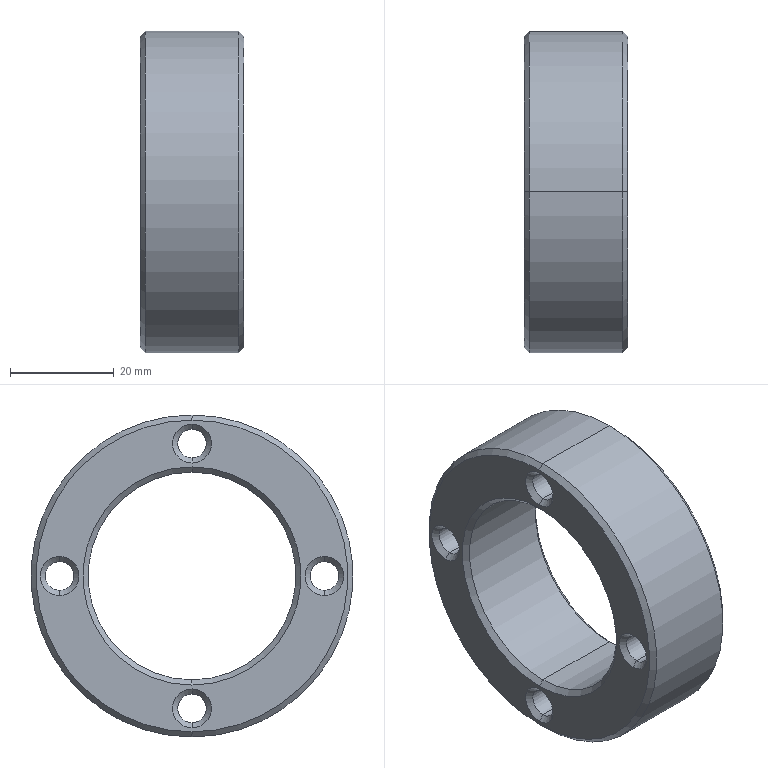Part | SolidWorks | features BaseBody 1 | 1 solid | 38 faces | box 20 x 62 x 62 mm | volume 32950 mm3 | cone 24 | cylinder 12 | plane 2 | commonest cylinder face diameters 5.5 x8 40 x2 62 x2
STEP:
#1=CARTESIAN_POINT('',(1.,0.,-28.25));
#2=VERTEX_POINT('',#1);
#3=CARTESIAN_POINT('',(1.,0.,-22.75));
#4=VERTEX_POINT('',#3);
#5=CARTESIAN_POINT('',(1.,0.,-25.5));
#6=DIRECTION('',(-1.,0.,0.));
#7=DIRECTION('',(0.,0.,-1.));
#8=AXIS2_PLACEMENT_3D('',#5,#6,#7);
#9=CIRCLE('',#8,2.75);
#10=EDGE_CURVE('',#2,#4,#9,.T.);
#11=ORIENTED_EDGE('',*,*,#10,.F.);
#12=CARTESIAN_POINT('',(0.,0.,-29.25));
#13=VERTEX_POINT('',#12);
#14=CARTESIAN_POINT('',(1.,0.,-28.25));
#15=DIRECTION('',(-0.7071,0.,-0.7071));
#16=VECTOR('',#15,1000.);
#17=LINE('',#14,#16);
#18=EDGE_CURVE('',#2,#13,#17,.T.);
#19=ORIENTED_EDGE('',*,*,#18,.T.);
#20=CARTESIAN_POINT('',(0.,0.,-21.75));
#21=VERTEX_POINT('',#20);
#22=CARTESIAN_POINT('',(0.,0.,-25.5));
#23=DIRECTION('',(1.,0.,0.));
#24=DIRECTION('',(0.,0.,-1.));
#25=AXIS2_PLACEMENT_3D('',#22,#23,#24);
#26=CIRCLE('',#25,3.75);
#27=EDGE_CURVE('',#21,#13,#26,.T.);
#28=ORIENTED_EDGE('',*,*,#27,.F.);
#29=CARTESIAN_POINT('',(1.,0.,-22.75));
#30=DIRECTION('',(-0.7071,0.,0.7071));
#31=VECTOR('',#30,1000.);
#32=LINE('',#29,#31);
#33=EDGE_CURVE('',#4,#21,#32,.T.);
#34=ORIENTED_EDGE('',*,*,#33,.F.);
#35=EDGE_LOOP('',(#11,#19,#28,#34));
#36=FACE_OUTER_BOUND('',#35,.T.);
#37=CARTESIAN_POINT('',(1.,0.,-25.5));
#38=DIRECTION('',(-1.,0.,0.));
#39=DIRECTION('',(0.,0.,1.));
#40=AXIS2_PLACEMENT_3D('',#37,#38,#39);
#41=CONICAL_SURFACE('',#40,2.75,0.7854);
#42=ADVANCED_FACE('',(#36),#41,.F.);
#43=CARTESIAN_POINT('',(1.,-25.5,-2.75));
#44=VERTEX_POINT('',#43);
#45=CARTESIAN_POINT('',(1.,-25.5,2.75));
#46=VERTEX_POINT('',#45);
#47=CARTESIAN_POINT('',(1.,-25.5,0.));
#48=DIRECTION('',(-1.,0.,0.));
#49=DIRECTION('',(0.,0.,-1.));
#50=AXIS2_PLACEMENT_3D('',#47,#48,#49);
#51=CIRCLE('',#50,2.75);
#52=EDGE_CURVE('',#44,#46,#51,.T.);
#53=ORIENTED_EDGE('',*,*,#52,.F.);
#54=CARTESIAN_POINT('',(0.,-25.5,-3.75));
#55=VERTEX_POINT('',#54);
#56=CARTESIAN_POINT('',(1.,-25.5,-2.75));
#57=DIRECTION('',(-0.7071,0.,-0.7071));
#58=VECTOR('',#57,1000.);
#59=LINE('',#56,#58);
#60=EDGE_CURVE('',#44,#55,#59,.T.);
#61=ORIENTED_EDGE('',*,*,#60,.T.);
#62=CARTESIAN_POINT('',(0.,-25.5,3.75));
#63=VERTEX_POINT('',#62);
#64=CARTESIAN_POINT('',(0.,-25.5,0.));
#65=DIRECTION('',(1.,0.,0.));
#66=DIRECTION('',(0.,0.,-1.));
#67=AXIS2_PLACEMENT_3D('',#64,#65,#66);
#68=CIRCLE('',#67,3.75);
#69=EDGE_CURVE('',#63,#55,#68,.T.);
#70=ORIENTED_EDGE('',*,*,#69,.F.);
#71=CARTESIAN_POINT('',(1.,-25.5,2.75));
#72=DIRECTION('',(-0.7071,0.,0.7071));
#73=VECTOR('',#72,1000.);
#74=LINE('',#71,#73);
#75=EDGE_CURVE('',#46,#63,#74,.T.);
#76=ORIENTED_EDGE('',*,*,#75,.F.);
#77=EDGE_LOOP('',(#53,#61,#70,#76));
#78=FACE_OUTER_BOUND('',#77,.T.);
#79=CARTESIAN_POINT('',(1.,-25.5,0.));
#80=DIRECTION('',(-1.,0.,0.));
#81=DIRECTION('',(0.,0.,1.));
#82=AXIS2_PLACEMENT_3D('',#79,#80,#81);
#83=CONICAL_SURFACE('',#82,2.75,0.7854);
#84=ADVANCED_FACE('',(#78),#83,.F.);
#85=CARTESIAN_POINT('',(1.,0.,22.75));
#86=VERTEX_POINT('',#85);
#87=CARTESIAN_POINT('',(1.,0.,28.25));
#88=VERTEX_POINT('',#87);
#89=CARTESIAN_POINT('',(1.,0.,25.5));
#90=DIRECTION('',(-1.,0.,0.));
#91=DIRECTION('',(0.,0.,-1.));
#92=AXIS2_PLACEMENT_3D('',#89,#90,#91);
#93=CIRCLE('',#92,2.75);
#94=EDGE_CURVE('',#86,#88,#93,.T.);
#95=ORIENTED_EDGE('',*,*,#94,.F.);
#96=CARTESIAN_POINT('',(0.,0.,21.75));
#97=VERTEX_POINT('',#96);
#98=CARTESIAN_POINT('',(1.,0.,22.75));
#99=DIRECTION('',(-0.7071,0.,-0.7071));
#100=VECTOR('',#99,1000.);
#101=LINE('',#98,#100);
#102=EDGE_CURVE('',#86,#97,#101,.T.);
#103=ORIENTED_EDGE('',*,*,#102,.T.);
#104=CARTESIAN_POINT('',(0.,0.,29.25));
#105=VERTEX_POINT('',#104);
#106=CARTESIAN_POINT('',(0.,0.,25.5));
#107=DIRECTION('',(1.,0.,0.));
#108=DIRECTION('',(0.,0.,-1.));
#109=AXIS2_PLACEMENT_3D('',#106,#107,#108);
#110=CIRCLE('',#109,3.75);
#111=EDGE_CURVE('',#105,#97,#110,.T.);
#112=ORIENTED_EDGE('',*,*,#111,.F.);
#113=CARTESIAN_POINT('',(1.,0.,28.25));
#114=DIRECTION('',(-0.7071,0.,0.7071));
#115=VECTOR('',#114,1000.);
#116=LINE('',#113,#115);
#117=EDGE_CURVE('',#88,#105,#116,.T.);
#118=ORIENTED_EDGE('',*,*,#117,.F.);
#119=EDGE_LOOP('',(#95,#103,#112,#118));
#120=FACE_OUTER_BOUND('',#119,.T.);
#121=CARTESIAN_POINT('',(1.,0.,25.5));
#122=DIRECTION('',(-1.,0.,0.));
#123=DIRECTION('',(0.,0.,1.));
#124=AXIS2_PLACEMENT_3D('',#121,#122,#123);
#125=CONICAL_SURFACE('',#124,2.75,0.7854);
#126=ADVANCED_FACE('',(#120),#125,.F.);
#127=CARTESIAN_POINT('',(1.,25.5,-2.75));
#128=VERTEX_POINT('',#127);
#129=CARTESIAN_POINT('',(1.,25.5,2.75));
#130=VERTEX_POINT('',#129);
#131=CARTESIAN_POINT('',(1.,25.5,0.));
#132=DIRECTION('',(-1.,0.,0.));
#133=DIRECTION('',(0.,0.,-1.));
#134=AXIS2_PLACEMENT_3D('',#131,#132,#133);
#135=CIRCLE('',#134,2.75);
#136=EDGE_CURVE('',#128,#130,#135,.T.);
#137=ORIENTED_EDGE('',*,*,#136,.F.);
#138=CARTESIAN_POINT('',(0.,25.5,-3.75));
#139=VERTEX_POINT('',#138);
#140=CARTESIAN_POINT('',(1.,25.5,-2.75));
#141=DIRECTION('',(-0.7071,0.,-0.7071));
#142=VECTOR('',#141,1000.);
#143=LINE('',#140,#142);
#144=EDGE_CURVE('',#128,#139,#143,.T.);
#145=ORIENTED_EDGE('',*,*,#144,.T.);
#146=CARTESIAN_POINT('',(0.,25.5,3.75));
#147=VERTEX_POINT('',#146);
#148=CARTESIAN_POINT('',(0.,25.5,0.));
#149=DIRECTION('',(1.,0.,0.));
#150=DIRECTION('',(0.,0.,-1.));
#151=AXIS2_PLACEMENT_3D('',#148,#149,#150);
#152=CIRCLE('',#151,3.75);
#153=EDGE_CURVE('',#147,#139,#152,.T.);
#154=ORIENTED_EDGE('',*,*,#153,.F.);
#155=CARTESIAN_POINT('',(1.,25.5,2.75));
#156=DIRECTION('',(-0.7071,0.,0.7071));
#157=VECTOR('',#156,1000.);
#158=LINE('',#155,#157);
#159=EDGE_CURVE('',#130,#147,#158,.T.);
#160=ORIENTED_EDGE('',*,*,#159,.F.);
#161=EDGE_LOOP('',(#137,#145,#154,#160));
#162=FACE_OUTER_BOUND('',#161,.T.);
#163=CARTESIAN_POINT('',(1.,25.5,0.));
#164=DIRECTION('',(-1.,0.,0.));
#165=DIRECTION('',(0.,0.,1.));
#166=AXIS2_PLACEMENT_3D('',#163,#164,#165);
#167=CONICAL_SURFACE('',#166,2.75,0.7854);
#168=ADVANCED_FACE('',(#162),#167,.F.);
#169=CARTESIAN_POINT('',(0.,0.,30.));
#170=VERTEX_POINT('',#169);
#171=CARTESIAN_POINT('',(0.,0.,-30.));
#172=VERTEX_POINT('',#171);
#173=CARTESIAN_POINT('',(0.,0.,0.));
#174=DIRECTION('',(-1.,0.,0.));
#175=DIRECTION('',(0.,0.,-1.));
#176=AXIS2_PLACEMENT_3D('',#173,#174,#175);
#177=CIRCLE('',#176,30.);
#178=EDGE_CURVE('',#170,#172,#177,.T.);
#179=ORIENTED_EDGE('',*,*,#178,.F.);
#180=CARTESIAN_POINT('',(1.,0.,31.));
#181=VERTEX_POINT('',#180);
#182=CARTESIAN_POINT('',(1.,0.,31.));
#183=DIRECTION('',(0.7071,0.,0.7071));
#184=VECTOR('',#183,1000.);
#185=LINE('',#182,#184);
#186=EDGE_CURVE('',#170,#181,#185,.T.);
#187=ORIENTED_EDGE('',*,*,#186,.T.);
#188=CARTESIAN_POINT('',(1.,0.,-31.));
#189=VERTEX_POINT('',#188);
#190=CARTESIAN_POINT('',(1.,0.,0.));
#191=DIRECTION('',(1.,0.,0.));
#192=DIRECTION('',(0.,0.,-1.));
#193=AXIS2_PLACEMENT_3D('',#190,#191,#192);
#194=CIRCLE('',#193,31.);
#195=EDGE_CURVE('',#189,#181,#194,.T.);
#196=ORIENTED_EDGE('',*,*,#195,.F.);
#197=CARTESIAN_POINT('',(1.,0.,-31.));
#198=DIRECTION('',(0.7071,0.,-0.7071));
#199=VECTOR('',#198,1000.);
#200=LINE('',#197,#199);
#201=EDGE_CURVE('',#172,#189,#200,.T.);
#202=ORIENTED_EDGE('',*,*,#201,.F.);
#203=EDGE_LOOP('',(#179,#187,#196,#202));
#204=FACE_OUTER_BOUND('',#203,.T.);
#205=CARTESIAN_POINT('',(1.,0.,0.));
#206=DIRECTION('',(1.,0.,0.));
#207=DIRECTION('',(0.,0.,-1.));
#208=AXIS2_PLACEMENT_3D('',#205,#206,#207);
#209=CONICAL_SURFACE('',#208,31.,0.7854);
#210=ADVANCED_FACE('',(#204),#209,.T.);
#211=CARTESIAN_POINT('',(1.,0.,-20.));
#212=VERTEX_POINT('',#211);
#213=CARTESIAN_POINT('',(1.,0.,20.));
#214=VERTEX_POINT('',#213);
#215=CARTESIAN_POINT('',(1.,0.,0.));
#216=DIRECTION('',(-1.,0.,0.));
#217=DIRECTION('',(0.,0.,-1.));
#218=AXIS2_PLACEMENT_3D('',#215,#216,#217);
#219=CIRCLE('',#218,20.);
#220=EDGE_CURVE('',#212,#214,#219,.T.);
#221=ORIENTED_EDGE('',*,*,#220,.F.);
#222=CARTESIAN_POINT('',(0.,0.,-21.));
#223=VERTEX_POINT('',#222);
#224=CARTESIAN_POINT('',(0.,0.,-21.));
#225=DIRECTION('',(-0.7071,0.,-0.7071));
#226=VECTOR('',#225,1000.);
#227=LINE('',#224,#226);
#228=EDGE_CURVE('',#212,#223,#227,.T.);
#229=ORIENTED_EDGE('',*,*,#228,.T.);
#230=CARTESIAN_POINT('',(0.,0.,21.));
#231=VERTEX_POINT('',#230);
#232=CARTESIAN_POINT('',(0.,0.,0.));
#233=DIRECTION('',(1.,0.,0.));
#234=DIRECTION('',(0.,0.,-1.));
#235=AXIS2_PLACEMENT_3D('',#232,#233,#234);
#236=CIRCLE('',#235,21.);
#237=EDGE_CURVE('',#231,#223,#236,.T.);
#238=ORIENTED_EDGE('',*,*,#237,.F.);
#239=CARTESIAN_POINT('',(0.,0.,21.));
#240=DIRECTION('',(-0.7071,0.,0.7071));
#241=VECTOR('',#240,1000.);
#242=LINE('',#239,#241);
#243=EDGE_CURVE('',#214,#231,#242,.T.);
#244=ORIENTED_EDGE('',*,*,#243,.F.);
#245=EDGE_LOOP('',(#221,#229,#238,#244));
#246=FACE_OUTER_BOUND('',#245,.T.);
#247=CARTESIAN_POINT('',(0.,0.,0.));
#248=DIRECTION('',(-1.,0.,0.));
#249=DIRECTION('',(0.,0.,1.));
#250=AXIS2_PLACEMENT_3D('',#247,#248,#249);
#251=CONICAL_SURFACE('',#250,21.,0.7854);
#252=ADVANCED_FACE('',(#246),#251,.F.);
#253=CARTESIAN_POINT('',(19.,0.,-22.75));
#254=VERTEX_POINT('',#253);
#255=CARTESIAN_POINT('',(19.,0.,-28.25));
#256=VERTEX_POINT('',#255);
#257=CARTESIAN_POINT('',(19.,0.,-25.5));
#258=DIRECTION('',(1.,0.,0.));
#259=DIRECTION('',(0.,0.,-1.));
#260=AXIS2_PLACEMENT_3D('',#257,#258,#259);
#261=CIRCLE('',#260,2.75);
#262=EDGE_CURVE('',#254,#256,#261,.T.);
#263=ORIENTED_EDGE('',*,*,#262,.F.);
#264=CARTESIAN_POINT('',(20.,0.,-21.75));
#265=VERTEX_POINT('',#264);
#266=CARTESIAN_POINT('',(20.,0.,-21.75));
#267=DIRECTION('',(0.7071,0.,0.7071));
#268=VECTOR('',#267,1000.);
#269=LINE('',#266,#268);
#270=EDGE_CURVE('',#254,#265,#269,.T.);
#271=ORIENTED_EDGE('',*,*,#270,.T.);
#272=CARTESIAN_POINT('',(20.,0.,-29.25));
#273=VERTEX_POINT('',#272);
#274=CARTESIAN_POINT('',(20.,0.,-25.5));
#275=DIRECTION('',(-1.,0.,0.));
#276=DIRECTION('',(0.,0.,-1.));
#277=AXIS2_PLACEMENT_3D('',#274,#275,#276);
#278=CIRCLE('',#277,3.75);
#279=EDGE_CURVE('',#273,#265,#278,.T.);
#280=ORIENTED_EDGE('',*,*,#279,.F.);
#281=CARTESIAN_POINT('',(20.,0.,-29.25));
#282=DIRECTION('',(0.7071,0.,-0.7071));
#283=VECTOR('',#282,1000.);
#284=LINE('',#281,#283);
#285=EDGE_CURVE('',#256,#273,#284,.T.);
#286=ORIENTED_EDGE('',*,*,#285,.F.);
#287=EDGE_LOOP('',(#263,#271,#280,#286));
#288=FACE_OUTER_BOUND('',#287,.T.);
#289=CARTESIAN_POINT('',(20.,0.,-25.5));
#290=DIRECTION('',(1.,0.,0.));
#291=DIRECTION('',(0.,0.,-1.));
#292=AXIS2_PLACEMENT_3D('',#289,#290,#291);
#293=CONICAL_SURFACE('',#292,3.75,0.7854);
#294=ADVANCED_FACE('',(#288),#293,.F.);
#295=CARTESIAN_POINT('',(19.,-25.5,2.75));
#296=VERTEX_POINT('',#295);
#297=CARTESIAN_POINT('',(19.,-25.5,-2.75));
#298=VERTEX_POINT('',#297);
#299=CARTESIAN_POINT('',(19.,-25.5,0.));
#300=DIRECTION('',(1.,0.,0.));
#301=DIRECTION('',(0.,0.,-1.));
#302=AXIS2_PLACEMENT_3D('',#299,#300,#301);
#303=CIRCLE('',#302,2.75);
#304=EDGE_CURVE('',#296,#298,#303,.T.);
#305=ORIENTED_EDGE('',*,*,#304,.F.);
#306=CARTESIAN_POINT('',(20.,-25.5,3.75));
#307=VERTEX_POINT('',#306);
#308=CARTESIAN_POINT('',(20.,-25.5,3.75));
#309=DIRECTION('',(0.7071,0.,0.7071));
#310=VECTOR('',#309,1000.);
#311=LINE('',#308,#310);
#312=EDGE_CURVE('',#296,#307,#311,.T.);
#313=ORIENTED_EDGE('',*,*,#312,.T.);
#314=CARTESIAN_POINT('',(20.,-25.5,-3.75));
#315=VERTEX_POINT('',#314);
#316=CARTESIAN_POINT('',(20.,-25.5,0.));
#317=DIRECTION('',(-1.,0.,0.));
#318=DIRECTION('',(0.,0.,-1.));
#319=AXIS2_PLACEMENT_3D('',#316,#317,#318);
#320=CIRCLE('',#319,3.75);
#321=EDGE_CURVE('',#315,#307,#320,.T.);
#322=ORIENTED_EDGE('',*,*,#321,.F.);
#323=CARTESIAN_POINT('',(20.,-25.5,-3.75));
#324=DIRECTION('',(0.7071,0.,-0.7071));
#325=VECTOR('',#324,1000.);
#326=LINE('',#323,#325);
#327=EDGE_CURVE('',#298,#315,#326,.T.);
#328=ORIENTED_EDGE('',*,*,#327,.F.);
#329=EDGE_LOOP('',(#305,#313,#322,#328));
#330=FACE_OUTER_BOUND('',#329,.T.);
#331=CARTESIAN_POINT('',(20.,-25.5,0.));
#332=DIRECTION('',(1.,0.,0.));
#333=DIRECTION('',(0.,0.,-1.));
#334=AXIS2_PLACEMENT_3D('',#331,#332,#333);
#335=CONICAL_SURFACE('',#334,3.75,0.7854);
#336=ADVANCED_FACE('',(#330),#335,.F.);
#337=CARTESIAN_POINT('',(19.,0.,28.25));
#338=VERTEX_POINT('',#337);
#339=CARTESIAN_POINT('',(19.,0.,22.75));
#340=VERTEX_POINT('',#339);
#341=CARTESIAN_POINT('',(19.,0.,25.5));
#342=DIRECTION('',(1.,0.,0.));
#343=DIRECTION('',(0.,0.,-1.));
#344=AXIS2_PLACEMENT_3D('',#341,#342,#343);
#345=CIRCLE('',#344,2.75);
#346=EDGE_CURVE('',#338,#340,#345,.T.);
#347=ORIENTED_EDGE('',*,*,#346,.F.);
#348=CARTESIAN_POINT('',(20.,0.,29.25));
#349=VERTEX_POINT('',#348);
#350=CARTESIAN_POINT('',(20.,0.,29.25));
#351=DIRECTION('',(0.7071,0.,0.7071));
#352=VECTOR('',#351,1000.);
#353=LINE('',#350,#352);
#354=EDGE_CURVE('',#338,#349,#353,.T.);
#355=ORIENTED_EDGE('',*,*,#354,.T.);
#356=CARTESIAN_POINT('',(20.,0.,21.75));
#357=VERTEX_POINT('',#356);
#358=CARTESIAN_POINT('',(20.,0.,25.5));
#359=DIRECTION('',(-1.,0.,0.));
#360=DIRECTION('',(0.,0.,-1.));
#361=AXIS2_PLACEMENT_3D('',#358,#359,#360);
#362=CIRCLE('',#361,3.75);
#363=EDGE_CURVE('',#357,#349,#362,.T.);
#364=ORIENTED_EDGE('',*,*,#363,.F.);
#365=CARTESIAN_POINT('',(20.,0.,21.75));
#366=DIRECTION('',(0.7071,0.,-0.7071));
#367=VECTOR('',#366,1000.);
#368=LINE('',#365,#367);
#369=EDGE_CURVE('',#340,#357,#368,.T.);
#370=ORIENTED_EDGE('',*,*,#369,.F.);
#371=EDGE_LOOP('',(#347,#355,#364,#370));
#372=FACE_OUTER_BOUND('',#371,.T.);
#373=CARTESIAN_POINT('',(20.,0.,25.5));
#374=DIRECTION('',(1.,0.,0.));
#375=DIRECTION('',(0.,0.,-1.));
#376=AXIS2_PLACEMENT_3D('',#373,#374,#375);
#377=CONICAL_SURFACE('',#376,3.75,0.7854);
#378=ADVANCED_FACE('',(#372),#377,.F.);
#379=CARTESIAN_POINT('',(19.,25.5,2.75));
#380=VERTEX_POINT('',#379);
#381=CARTESIAN_POINT('',(19.,25.5,-2.75));
#382=VERTEX_POINT('',#381);
#383=CARTESIAN_POINT('',(19.,25.5,0.));
#384=DIRECTION('',(1.,0.,0.));
#385=DIRECTION('',(0.,0.,-1.));
#386=AXIS2_PLACEMENT_3D('',#383,#384,#385);
#387=CIRCLE('',#386,2.75);
#388=EDGE_CURVE('',#380,#382,#387,.T.);
#389=ORIENTED_EDGE('',*,*,#388,.F.);
#390=CARTESIAN_POINT('',(20.,25.5,3.75));
#391=VERTEX_POINT('',#390);
#392=CARTESIAN_POINT('',(20.,25.5,3.75));
#393=DIRECTION('',(0.7071,0.,0.7071));
#394=VECTOR('',#393,1000.);
#395=LINE('',#392,#394);
#396=EDGE_CURVE('',#380,#391,#395,.T.);
#397=ORIENTED_EDGE('',*,*,#396,.T.);
#398=CARTESIAN_POINT('',(20.,25.5,-3.75));
#399=VERTEX_POINT('',#398);
#400=CARTESIAN_POINT('',(20.,25.5,0.));
#401=DIRECTION('',(-1.,0.,0.));
#402=DIRECTION('',(0.,0.,-1.));
#403=AXIS2_PLACEMENT_3D('',#400,#401,#402);
#404=CIRCLE('',#403,3.75);
#405=EDGE_CURVE('',#399,#391,#404,.T.);
#406=ORIENTED_EDGE('',*,*,#405,.F.);
#407=CARTESIAN_POINT('',(20.,25.5,-3.75));
#408=DIRECTION('',(0.7071,0.,-0.7071));
#409=VECTOR('',#408,1000.);
#410=LINE('',#407,#409);
#411=EDGE_CURVE('',#382,#399,#410,.T.);
#412=ORIENTED_EDGE('',*,*,#411,.F.);
#413=EDGE_LOOP('',(#389,#397,#406,#412));
#414=FACE_OUTER_BOUND('',#413,.T.);
#415=CARTESIAN_POINT('',(20.,25.5,0.));
#416=DIRECTION('',(1.,0.,0.));
#417=DIRECTION('',(0.,0.,-1.));
#418=AXIS2_PLACEMENT_3D('',#415,#416,#417);
#419=CONICAL_SURFACE('',#418,3.75,0.7854);
#420=ADVANCED_FACE('',(#414),#419,.F.);
#421=CARTESIAN_POINT('',(20.,0.,-30.));
#422=VERTEX_POINT('',#421);
#423=CARTESIAN_POINT('',(20.,0.,30.));
#424=VERTEX_POINT('',#423);
#425=CARTESIAN_POINT('',(20.,0.,0.));
#426=DIRECTION('',(1.,0.,0.));
#427=DIRECTION('',(0.,0.,-1.));
#428=AXIS2_PLACEMENT_3D('',#425,#426,#427);
#429=CIRCLE('',#428,30.);
#430=EDGE_CURVE('',#422,#424,#429,.T.);
#431=ORIENTED_EDGE('',*,*,#430,.F.);
#432=CARTESIAN_POINT('',(19.,0.,-31.));
#433=VERTEX_POINT('',#432);
#434=CARTESIAN_POINT('',(20.,0.,-30.));
#435=DIRECTION('',(-0.7071,0.,-0.7071));
#436=VECTOR('',#435,1000.);
#437=LINE('',#434,#436);
#438=EDGE_CURVE('',#422,#433,#437,.T.);
#439=ORIENTED_EDGE('',*,*,#438,.T.);
#440=CARTESIAN_POINT('',(19.,0.,31.));
#441=VERTEX_POINT('',#440);
#442=CARTESIAN_POINT('',(19.,0.,0.));
#443=DIRECTION('',(-1.,0.,0.));
#444=DIRECTION('',(0.,0.,-1.));
#445=AXIS2_PLACEMENT_3D('',#442,#443,#444);
#446=CIRCLE('',#445,31.);
#447=EDGE_CURVE('',#441,#433,#446,.T.);
#448=ORIENTED_EDGE('',*,*,#447,.F.);
#449=CARTESIAN_POINT('',(20.,0.,30.));
#450=DIRECTION('',(-0.7071,0.,0.7071));
#451=VECTOR('',#450,1000.);
#452=LINE('',#449,#451);
#453=EDGE_CURVE('',#424,#441,#452,.T.);
#454=ORIENTED_EDGE('',*,*,#453,.F.);
#455=EDGE_LOOP('',(#431,#439,#448,#454));
#456=FACE_OUTER_BOUND('',#455,.T.);
#457=CARTESIAN_POINT('',(20.,0.,0.));
#458=DIRECTION('',(-1.,0.,0.));
#459=DIRECTION('',(0.,0.,1.));
#460=AXIS2_PLACEMENT_3D('',#457,#458,#459);
#461=CONICAL_SURFACE('',#460,30.,0.7854);
#462=ADVANCED_FACE('',(#456),#461,.T.);
#463=CARTESIAN_POINT('',(19.,0.,20.));
#464=VERTEX_POINT('',#463);
#465=CARTESIAN_POINT('',(19.,0.,-20.));
#466=VERTEX_POINT('',#465);
#467=CARTESIAN_POINT('',(19.,0.,0.));
#468=DIRECTION('',(1.,0.,0.));
#469=DIRECTION('',(0.,0.,-1.));
#470=AXIS2_PLACEMENT_3D('',#467,#468,#469);
#471=CIRCLE('',#470,20.);
#472=EDGE_CURVE('',#464,#466,#471,.T.);
#473=ORIENTED_EDGE('',*,*,#472,.F.);
#474=CARTESIAN_POINT('',(20.,0.,21.));
#475=VERTEX_POINT('',#474);
#476=CARTESIAN_POINT('',(19.,0.,20.));
#477=DIRECTION('',(0.7071,0.,0.7071));
#478=VECTOR('',#477,1000.);
#479=LINE('',#476,#478);
#480=EDGE_CURVE('',#464,#475,#479,.T.);
#481=ORIENTED_EDGE('',*,*,#480,.T.);
#482=CARTESIAN_POINT('',(20.,0.,-21.));
#483=VERTEX_POINT('',#482);
#484=CARTESIAN_POINT('',(20.,0.,0.));
#485=DIRECTION('',(-1.,0.,0.));
#486=DIRECTION('',(0.,0.,-1.));
#487=AXIS2_PLACEMENT_3D('',#484,#485,#486);
#488=CIRCLE('',#487,21.);
#489=EDGE_CURVE('',#483,#475,#488,.T.);
#490=ORIENTED_EDGE('',*,*,#489,.F.);
#491=CARTESIAN_POINT('',(19.,0.,-20.));
#492=DIRECTION('',(0.7071,0.,-0.7071));
#493=VECTOR('',#492,1000.);
#494=LINE('',#491,#493);
#495=EDGE_CURVE('',#466,#483,#494,.T.);
#496=ORIENTED_EDGE('',*,*,#495,.F.);
#497=EDGE_LOOP('',(#473,#481,#490,#496));
#498=FACE_OUTER_BOUND('',#497,.T.);
#499=CARTESIAN_POINT('',(19.,0.,0.));
#500=DIRECTION('',(1.,0.,0.));
#501=DIRECTION('',(0.,0.,-1.));
#502=AXIS2_PLACEMENT_3D('',#499,#500,#501);
#503=CONICAL_SURFACE('',#502,20.,0.7854);
#504=ADVANCED_FACE('',(#498),#503,.F.);
#505=ORIENTED_EDGE('',*,*,#262,.T.);
#506=CARTESIAN_POINT('',(0.,0.,-28.25));
#507=DIRECTION('',(-1.,0.,0.));
#508=VECTOR('',#507,1000.);
#509=LINE('',#506,#508);
#510=EDGE_CURVE('',#256,#2,#509,.T.);
#511=ORIENTED_EDGE('',*,*,#510,.T.);
#512=ORIENTED_EDGE('',*,*,#10,.T.);
#513=CARTESIAN_POINT('',(0.,0.,-22.75));
#514=DIRECTION('',(-1.,0.,0.));
#515=VECTOR('',#514,1000.);
#516=LINE('',#513,#515);
#517=EDGE_CURVE('',#254,#4,#516,.T.);
#518=ORIENTED_EDGE('',*,*,#517,.F.);
#519=EDGE_LOOP('',(#505,#511,#512,#518));
#520=FACE_OUTER_BOUND('',#519,.T.);
#521=CARTESIAN_POINT('',(0.,0.,-25.5));
#522=DIRECTION('',(-1.,0.,0.));
#523=DIRECTION('',(0.,0.,1.));
#524=AXIS2_PLACEMENT_3D('',#521,#522,#523);
#525=CYLINDRICAL_SURFACE('',#524,2.75);
#526=ADVANCED_FACE('',(#520),#525,.F.);
#527=ORIENTED_EDGE('',*,*,#304,.T.);
#528=CARTESIAN_POINT('',(0.,-25.5,-2.75));
#529=DIRECTION('',(-1.,0.,0.));
#530=VECTOR('',#529,1000.);
#531=LINE('',#528,#530);
#532=EDGE_CURVE('',#298,#44,#531,.T.);
#533=ORIENTED_EDGE('',*,*,#532,.T.);
#534=ORIENTED_EDGE('',*,*,#52,.T.);
#535=CARTESIAN_POINT('',(0.,-25.5,2.75));
#536=DIRECTION('',(-1.,0.,0.));
#537=VECTOR('',#536,1000.);
#538=LINE('',#535,#537);
#539=EDGE_CURVE('',#296,#46,#538,.T.);
#540=ORIENTED_EDGE('',*,*,#539,.F.);
#541=EDGE_LOOP('',(#527,#533,#534,#540));
#542=FACE_OUTER_BOUND('',#541,.T.);
#543=CARTESIAN_POINT('',(0.,-25.5,0.));
#544=DIRECTION('',(-1.,0.,0.));
#545=DIRECTION('',(0.,0.,1.));
#546=AXIS2_PLACEMENT_3D('',#543,#544,#545);
#547=CYLINDRICAL_SURFACE('',#546,2.75);
#548=ADVANCED_FACE('',(#542),#547,.F.);
#549=ORIENTED_EDGE('',*,*,#346,.T.);
#550=CARTESIAN_POINT('',(0.,0.,22.75));
#551=DIRECTION('',(-1.,0.,0.));
#552=VECTOR('',#551,1000.);
#553=LINE('',#550,#552);
#554=EDGE_CURVE('',#340,#86,#553,.T.);
#555=ORIENTED_EDGE('',*,*,#554,.T.);
#556=ORIENTED_EDGE('',*,*,#94,.T.);
#557=CARTESIAN_POINT('',(0.,0.,28.25));
#558=DIRECTION('',(-1.,0.,0.));
#559=VECTOR('',#558,1000.);
#560=LINE('',#557,#559);
#561=EDGE_CURVE('',#338,#88,#560,.T.);
#562=ORIENTED_EDGE('',*,*,#561,.F.);
#563=EDGE_LOOP('',(#549,#555,#556,#562));
#564=FACE_OUTER_BOUND('',#563,.T.);
#565=CARTESIAN_POINT('',(0.,0.,25.5));
#566=DIRECTION('',(-1.,0.,0.));
#567=DIRECTION('',(0.,0.,1.));
#568=AXIS2_PLACEMENT_3D('',#565,#566,#567);
#569=CYLINDRICAL_SURFACE('',#568,2.75);
#570=ADVANCED_FACE('',(#564),#569,.F.);
#571=ORIENTED_EDGE('',*,*,#388,.T.);
#572=CARTESIAN_POINT('',(0.,25.5,-2.75));
#573=DIRECTION('',(-1.,0.,0.));
#574=VECTOR('',#573,1000.);
#575=LINE('',#572,#574);
#576=EDGE_CURVE('',#382,#128,#575,.T.);
#577=ORIENTED_EDGE('',*,*,#576,.T.);
#578=ORIENTED_EDGE('',*,*,#136,.T.);
#579=CARTESIAN_POINT('',(0.,25.5,2.75));
#580=DIRECTION('',(-1.,0.,0.));
#581=VECTOR('',#580,1000.);
#582=LINE('',#579,#581);
#583=EDGE_CURVE('',#380,#130,#582,.T.);
#584=ORIENTED_EDGE('',*,*,#583,.F.);
#585=EDGE_LOOP('',(#571,#577,#578,#584));
#586=FACE_OUTER_BOUND('',#585,.T.);
#587=CARTESIAN_POINT('',(0.,25.5,0.));
#588=DIRECTION('',(-1.,0.,0.));
#589=DIRECTION('',(0.,0.,1.));
#590=AXIS2_PLACEMENT_3D('',#587,#588,#589);
#591=CYLINDRICAL_SURFACE('',#590,2.75);
#592=ADVANCED_FACE('',(#586),#591,.F.);
#593=ORIENTED_EDGE('',*,*,#472,.T.);
#594=CARTESIAN_POINT('',(20.,0.,-20.));
#595=DIRECTION('',(-1.,0.,0.));
#596=VECTOR('',#595,1000.);
#597=LINE('',#594,#596);
#598=EDGE_CURVE('',#466,#212,#597,.T.);
#599=ORIENTED_EDGE('',*,*,#598,.T.);
#600=ORIENTED_EDGE('',*,*,#220,.T.);
#601=CARTESIAN_POINT('',(20.,0.,20.));
#602=DIRECTION('',(-1.,0.,0.));
#603=VECTOR('',#602,1000.);
#604=LINE('',#601,#603);
#605=EDGE_CURVE('',#464,#214,#604,.T.);
#606=ORIENTED_EDGE('',*,*,#605,.F.);
#607=EDGE_LOOP('',(#593,#599,#600,#606));
#608=FACE_OUTER_BOUND('',#607,.T.);
#609=CARTESIAN_POINT('',(20.,0.,0.));
#610=DIRECTION('',(-1.,0.,0.));
#611=DIRECTION('',(0.,0.,1.));
#612=AXIS2_PLACEMENT_3D('',#609,#610,#611);
#613=CYLINDRICAL_SURFACE('',#612,20.);
#614=ADVANCED_FACE('',(#608),#613,.F.);
#615=ORIENTED_EDGE('',*,*,#447,.T.);
#616=CARTESIAN_POINT('',(20.,0.,-31.));
#617=DIRECTION('',(-1.,0.,0.));
#618=VECTOR('',#617,1000.);
#619=LINE('',#616,#618);
#620=EDGE_CURVE('',#433,#189,#619,.T.);
#621=ORIENTED_EDGE('',*,*,#620,.T.);
#622=ORIENTED_EDGE('',*,*,#195,.T.);
#623=CARTESIAN_POINT('',(20.,0.,31.));
#624=DIRECTION('',(-1.,0.,0.));
#625=VECTOR('',#624,1000.);
#626=LINE('',#623,#625);
#627=EDGE_CURVE('',#441,#181,#626,.T.);
#628=ORIENTED_EDGE('',*,*,#627,.F.);
#629=EDGE_LOOP('',(#615,#621,#622,#628));
#630=FACE_OUTER_BOUND('',#629,.T.);
#631=CARTESIAN_POINT('',(20.,0.,0.));
#632=DIRECTION('',(-1.,0.,0.));
#633=DIRECTION('',(0.,0.,1.));
#634=AXIS2_PLACEMENT_3D('',#631,#632,#633);
#635=CYLINDRICAL_SURFACE('',#634,31.);
#636=ADVANCED_FACE('',(#630),#635,.T.);
#637=ORIENTED_EDGE('',*,*,#489,.T.);
#638=CARTESIAN_POINT('',(20.,0.,0.));
#639=DIRECTION('',(-1.,0.,0.));
#640=DIRECTION('',(0.,0.,-1.));
#641=AXIS2_PLACEMENT_3D('',#638,#639,#640);
#642=CIRCLE('',#641,21.);
#643=EDGE_CURVE('',#475,#483,#642,.T.);
#644=ORIENTED_EDGE('',*,*,#643,.T.);
#645=EDGE_LOOP('',(#637,#644));
#646=FACE_BOUND('',#645,.T.);
#647=CARTESIAN_POINT('',(20.,0.,0.));
#648=DIRECTION('',(1.,0.,0.));
#649=DIRECTION('',(0.,0.,-1.));
#650=AXIS2_PLACEMENT_3D('',#647,#648,#649);
#651=CIRCLE('',#650,30.);
#652=EDGE_CURVE('',#424,#422,#651,.T.);
#653=ORIENTED_EDGE('',*,*,#652,.T.);
#654=ORIENTED_EDGE('',*,*,#430,.T.);
#655=EDGE_LOOP('',(#653,#654));
#656=FACE_OUTER_BOUND('',#655,.T.);
#657=ORIENTED_EDGE('',*,*,#405,.T.);
#658=CARTESIAN_POINT('',(20.,25.5,0.));
#659=DIRECTION('',(-1.,0.,0.));
#660=DIRECTION('',(0.,0.,-1.));
#661=AXIS2_PLACEMENT_3D('',#658,#659,#660);
#662=CIRCLE('',#661,3.75);
#663=EDGE_CURVE('',#391,#399,#662,.T.);
#664=ORIENTED_EDGE('',*,*,#663,.T.);
#665=EDGE_LOOP('',(#657,#664));
#666=FACE_BOUND('',#665,.T.);
#667=ORIENTED_EDGE('',*,*,#363,.T.);
#668=CARTESIAN_POINT('',(20.,0.,25.5));
#669=DIRECTION('',(-1.,0.,0.));
#670=DIRECTION('',(0.,0.,-1.));
#671=AXIS2_PLACEMENT_3D('',#668,#669,#670);
#672=CIRCLE('',#671,3.75);
#673=EDGE_CURVE('',#349,#357,#672,.T.);
#674=ORIENTED_EDGE('',*,*,#673,.T.);
#675=EDGE_LOOP('',(#667,#674));
#676=FACE_BOUND('',#675,.T.);
#677=ORIENTED_EDGE('',*,*,#321,.T.);
#678=CARTESIAN_POINT('',(20.,-25.5,0.));
#679=DIRECTION('',(-1.,0.,0.));
#680=DIRECTION('',(0.,0.,-1.));
#681=AXIS2_PLACEMENT_3D('',#678,#679,#680);
#682=CIRCLE('',#681,3.75);
#683=EDGE_CURVE('',#307,#315,#682,.T.);
#684=ORIENTED_EDGE('',*,*,#683,.T.);
#685=EDGE_LOOP('',(#677,#684));
#686=FACE_BOUND('',#685,.T.);
#687=ORIENTED_EDGE('',*,*,#279,.T.);
#688=CARTESIAN_POINT('',(20.,0.,-25.5));
#689=DIRECTION('',(-1.,0.,0.));
#690=DIRECTION('',(0.,0.,-1.));
#691=AXIS2_PLACEMENT_3D('',#688,#689,#690);
#692=CIRCLE('',#691,3.75);
#693=EDGE_CURVE('',#265,#273,#692,.T.);
#694=ORIENTED_EDGE('',*,*,#693,.T.);
#695=EDGE_LOOP('',(#687,#694));
#696=FACE_BOUND('',#695,.T.);
#697=CARTESIAN_POINT('',(20.,0.,0.));
#698=DIRECTION('',(1.,0.,0.));
#699=DIRECTION('',(0.,0.,-1.));
#700=AXIS2_PLACEMENT_3D('',#697,#698,#699);
#701=PLANE('',#700);
#702=ADVANCED_FACE('',(#646,#656,#666,#676,#686,#696),#701,.T.);
#703=ORIENTED_EDGE('',*,*,#237,.T.);
#704=CARTESIAN_POINT('',(0.,0.,0.));
#705=DIRECTION('',(1.,0.,0.));
#706=DIRECTION('',(0.,0.,-1.));
#707=AXIS2_PLACEMENT_3D('',#704,#705,#706);
#708=CIRCLE('',#707,21.);
#709=EDGE_CURVE('',#223,#231,#708,.T.);
#710=ORIENTED_EDGE('',*,*,#709,.T.);
#711=EDGE_LOOP('',(#703,#710));
#712=FACE_BOUND('',#711,.T.);
#713=CARTESIAN_POINT('',(0.,0.,0.));
#714=DIRECTION('',(-1.,0.,0.));
#715=DIRECTION('',(0.,0.,-1.));
#716=AXIS2_PLACEMENT_3D('',#713,#714,#715);
#717=CIRCLE('',#716,30.);
#718=EDGE_CURVE('',#172,#170,#717,.T.);
#719=ORIENTED_EDGE('',*,*,#718,.T.);
#720=ORIENTED_EDGE('',*,*,#178,.T.);
#721=EDGE_LOOP('',(#719,#720));
#722=FACE_OUTER_BOUND('',#721,.T.);
#723=ORIENTED_EDGE('',*,*,#153,.T.);
#724=CARTESIAN_POINT('',(0.,25.5,0.));
#725=DIRECTION('',(1.,0.,0.));
#726=DIRECTION('',(0.,0.,-1.));
#727=AXIS2_PLACEMENT_3D('',#724,#725,#726);
#728=CIRCLE('',#727,3.75);
#729=EDGE_CURVE('',#139,#147,#728,.T.);
#730=ORIENTED_EDGE('',*,*,#729,.T.);
#731=EDGE_LOOP('',(#723,#730));
#732=FACE_BOUND('',#731,.T.);
#733=ORIENTED_EDGE('',*,*,#111,.T.);
#734=CARTESIAN_POINT('',(0.,0.,25.5));
#735=DIRECTION('',(1.,0.,0.));
#736=DIRECTION('',(0.,0.,-1.));
#737=AXIS2_PLACEMENT_3D('',#734,#735,#736);
#738=CIRCLE('',#737,3.75);
#739=EDGE_CURVE('',#97,#105,#738,.T.);
#740=ORIENTED_EDGE('',*,*,#739,.T.);
#741=EDGE_LOOP('',(#733,#740));
#742=FACE_BOUND('',#741,.T.);
#743=ORIENTED_EDGE('',*,*,#69,.T.);
#744=CARTESIAN_POINT('',(0.,-25.5,0.));
#745=DIRECTION('',(1.,0.,0.));
#746=DIRECTION('',(0.,0.,-1.));
#747=AXIS2_PLACEMENT_3D('',#744,#745,#746);
#748=CIRCLE('',#747,3.75);
#749=EDGE_CURVE('',#55,#63,#748,.T.);
#750=ORIENTED_EDGE('',*,*,#749,.T.);
#751=EDGE_LOOP('',(#743,#750));
#752=FACE_BOUND('',#751,.T.);
#753=ORIENTED_EDGE('',*,*,#27,.T.);
#754=CARTESIAN_POINT('',(0.,0.,-25.5));
#755=DIRECTION('',(1.,0.,0.));
#756=DIRECTION('',(0.,0.,-1.));
#757=AXIS2_PLACEMENT_3D('',#754,#755,#756);
#758=CIRCLE('',#757,3.75);
#759=EDGE_CURVE('',#13,#21,#758,.T.);
#760=ORIENTED_EDGE('',*,*,#759,.T.);
#761=EDGE_LOOP('',(#753,#760));
#762=FACE_BOUND('',#761,.T.);
#763=CARTESIAN_POINT('',(0.,0.,0.));
#764=DIRECTION('',(1.,0.,0.));
#765=DIRECTION('',(0.,0.,-1.));
#766=AXIS2_PLACEMENT_3D('',#763,#764,#765);
#767=PLANE('',#766);
#768=ADVANCED_FACE('',(#712,#722,#732,#742,#752,#762),#767,.F.);
#769=ORIENTED_EDGE('',*,*,#620,.F.);
#770=CARTESIAN_POINT('',(19.,0.,0.));
#771=DIRECTION('',(-1.,0.,0.));
#772=DIRECTION('',(0.,0.,-1.));
#773=AXIS2_PLACEMENT_3D('',#770,#771,#772);
#774=CIRCLE('',#773,31.);
#775=EDGE_CURVE('',#433,#441,#774,.T.);
#776=ORIENTED_EDGE('',*,*,#775,.T.);
#777=ORIENTED_EDGE('',*,*,#627,.T.);
#778=CARTESIAN_POINT('',(1.,0.,0.));
#779=DIRECTION('',(1.,0.,0.));
#780=DIRECTION('',(0.,0.,-1.));
#781=AXIS2_PLACEMENT_3D('',#778,#779,#780);
#782=CIRCLE('',#781,31.);
#783=EDGE_CURVE('',#181,#189,#782,.T.);
#784=ORIENTED_EDGE('',*,*,#783,.T.);
#785=EDGE_LOOP('',(#769,#776,#777,#784));
#786=FACE_OUTER_BOUND('',#785,.T.);
#787=CARTESIAN_POINT('',(20.,0.,0.));
#788=DIRECTION('',(-1.,0.,0.));
#789=DIRECTION('',(0.,0.,1.));
#790=AXIS2_PLACEMENT_3D('',#787,#788,#789);
#791=CYLINDRICAL_SURFACE('',#790,31.);
#792=ADVANCED_FACE('',(#786),#791,.T.);
#793=ORIENTED_EDGE('',*,*,#598,.F.);
#794=CARTESIAN_POINT('',(19.,0.,0.));
#795=DIRECTION('',(1.,0.,0.));
#796=DIRECTION('',(0.,0.,-1.));
#797=AXIS2_PLACEMENT_3D('',#794,#795,#796);
#798=CIRCLE('',#797,20.);
#799=EDGE_CURVE('',#466,#464,#798,.T.);
#800=ORIENTED_EDGE('',*,*,#799,.T.);
#801=ORIENTED_EDGE('',*,*,#605,.T.);
#802=CARTESIAN_POINT('',(1.,0.,0.));
#803=DIRECTION('',(-1.,0.,0.));
#804=DIRECTION('',(0.,0.,-1.));
#805=AXIS2_PLACEMENT_3D('',#802,#803,#804);
#806=CIRCLE('',#805,20.);
#807=EDGE_CURVE('',#214,#212,#806,.T.);
#808=ORIENTED_EDGE('',*,*,#807,.T.);
#809=EDGE_LOOP('',(#793,#800,#801,#808));
#810=FACE_OUTER_BOUND('',#809,.T.);
#811=CARTESIAN_POINT('',(20.,0.,0.));
#812=DIRECTION('',(-1.,0.,0.));
#813=DIRECTION('',(0.,0.,1.));
#814=AXIS2_PLACEMENT_3D('',#811,#812,#813);
#815=CYLINDRICAL_SURFACE('',#814,20.);
#816=ADVANCED_FACE('',(#810),#815,.F.);
#817=ORIENTED_EDGE('',*,*,#576,.F.);
#818=CARTESIAN_POINT('',(19.,25.5,0.));
#819=DIRECTION('',(1.,0.,0.));
#820=DIRECTION('',(0.,0.,-1.));
#821=AXIS2_PLACEMENT_3D('',#818,#819,#820);
#822=CIRCLE('',#821,2.75);
#823=EDGE_CURVE('',#382,#380,#822,.T.);
#824=ORIENTED_EDGE('',*,*,#823,.T.);
#825=ORIENTED_EDGE('',*,*,#583,.T.);
#826=CARTESIAN_POINT('',(1.,25.5,0.));
#827=DIRECTION('',(-1.,0.,0.));
#828=DIRECTION('',(0.,0.,-1.));
#829=AXIS2_PLACEMENT_3D('',#826,#827,#828);
#830=CIRCLE('',#829,2.75);
#831=EDGE_CURVE('',#130,#128,#830,.T.);
#832=ORIENTED_EDGE('',*,*,#831,.T.);
#833=EDGE_LOOP('',(#817,#824,#825,#832));
#834=FACE_OUTER_BOUND('',#833,.T.);
#835=CARTESIAN_POINT('',(0.,25.5,0.));
#836=DIRECTION('',(-1.,0.,0.));
#837=DIRECTION('',(0.,0.,1.));
#838=AXIS2_PLACEMENT_3D('',#835,#836,#837);
#839=CYLINDRICAL_SURFACE('',#838,2.75);
#840=ADVANCED_FACE('',(#834),#839,.F.);
#841=ORIENTED_EDGE('',*,*,#554,.F.);
#842=CARTESIAN_POINT('',(19.,0.,25.5));
#843=DIRECTION('',(1.,0.,0.));
#844=DIRECTION('',(0.,0.,-1.));
#845=AXIS2_PLACEMENT_3D('',#842,#843,#844);
#846=CIRCLE('',#845,2.75);
#847=EDGE_CURVE('',#340,#338,#846,.T.);
#848=ORIENTED_EDGE('',*,*,#847,.T.);
#849=ORIENTED_EDGE('',*,*,#561,.T.);
#850=CARTESIAN_POINT('',(1.,0.,25.5));
#851=DIRECTION('',(-1.,0.,0.));
#852=DIRECTION('',(0.,0.,-1.));
#853=AXIS2_PLACEMENT_3D('',#850,#851,#852);
#854=CIRCLE('',#853,2.75);
#855=EDGE_CURVE('',#88,#86,#854,.T.);
#856=ORIENTED_EDGE('',*,*,#855,.T.);
#857=EDGE_LOOP('',(#841,#848,#849,#856));
#858=FACE_OUTER_BOUND('',#857,.T.);
#859=CARTESIAN_POINT('',(0.,0.,25.5));
#860=DIRECTION('',(-1.,0.,0.));
#861=DIRECTION('',(0.,0.,1.));
#862=AXIS2_PLACEMENT_3D('',#859,#860,#861);
#863=CYLINDRICAL_SURFACE('',#862,2.75);
#864=ADVANCED_FACE('',(#858),#863,.F.);
#865=ORIENTED_EDGE('',*,*,#532,.F.);
#866=CARTESIAN_POINT('',(19.,-25.5,0.));
#867=DIRECTION('',(1.,0.,0.));
#868=DIRECTION('',(0.,0.,-1.));
#869=AXIS2_PLACEMENT_3D('',#866,#867,#868);
#870=CIRCLE('',#869,2.75);
#871=EDGE_CURVE('',#298,#296,#870,.T.);
#872=ORIENTED_EDGE('',*,*,#871,.T.);
#873=ORIENTED_EDGE('',*,*,#539,.T.);
#874=CARTESIAN_POINT('',(1.,-25.5,0.));
#875=DIRECTION('',(-1.,0.,0.));
#876=DIRECTION('',(0.,0.,-1.));
#877=AXIS2_PLACEMENT_3D('',#874,#875,#876);
#878=CIRCLE('',#877,2.75);
#879=EDGE_CURVE('',#46,#44,#878,.T.);
#880=ORIENTED_EDGE('',*,*,#879,.T.);
#881=EDGE_LOOP('',(#865,#872,#873,#880));
#882=FACE_OUTER_BOUND('',#881,.T.);
#883=CARTESIAN_POINT('',(0.,-25.5,0.));
#884=DIRECTION('',(-1.,0.,0.));
#885=DIRECTION('',(0.,0.,1.));
#886=AXIS2_PLACEMENT_3D('',#883,#884,#885);
#887=CYLINDRICAL_SURFACE('',#886,2.75);
#888=ADVANCED_FACE('',(#882),#887,.F.);
#889=ORIENTED_EDGE('',*,*,#510,.F.);
#890=CARTESIAN_POINT('',(19.,0.,-25.5));
#891=DIRECTION('',(1.,0.,0.));
#892=DIRECTION('',(0.,0.,-1.));
#893=AXIS2_PLACEMENT_3D('',#890,#891,#892);
#894=CIRCLE('',#893,2.75);
#895=EDGE_CURVE('',#256,#254,#894,.T.);
#896=ORIENTED_EDGE('',*,*,#895,.T.);
#897=ORIENTED_EDGE('',*,*,#517,.T.);
#898=CARTESIAN_POINT('',(1.,0.,-25.5));
#899=DIRECTION('',(-1.,0.,0.));
#900=DIRECTION('',(0.,0.,-1.));
#901=AXIS2_PLACEMENT_3D('',#898,#899,#900);
#902=CIRCLE('',#901,2.75);
#903=EDGE_CURVE('',#4,#2,#902,.T.);
#904=ORIENTED_EDGE('',*,*,#903,.T.);
#905=EDGE_LOOP('',(#889,#896,#897,#904));
#906=FACE_OUTER_BOUND('',#905,.T.);
#907=CARTESIAN_POINT('',(0.,0.,-25.5));
#908=DIRECTION('',(-1.,0.,0.));
#909=DIRECTION('',(0.,0.,1.));
#910=AXIS2_PLACEMENT_3D('',#907,#908,#909);
#911=CYLINDRICAL_SURFACE('',#910,2.75);
#912=ADVANCED_FACE('',(#906),#911,.F.);
#913=ORIENTED_EDGE('',*,*,#480,.F.);
#914=ORIENTED_EDGE('',*,*,#799,.F.);
#915=ORIENTED_EDGE('',*,*,#495,.T.);
#916=ORIENTED_EDGE('',*,*,#643,.F.);
#917=EDGE_LOOP('',(#913,#914,#915,#916));
#918=FACE_OUTER_BOUND('',#917,.T.);
#919=CARTESIAN_POINT('',(19.,0.,0.));
#920=DIRECTION('',(1.,0.,0.));
#921=DIRECTION('',(0.,0.,-1.));
#922=AXIS2_PLACEMENT_3D('',#919,#920,#921);
#923=CONICAL_SURFACE('',#922,20.,0.7854);
#924=ADVANCED_FACE('',(#918),#923,.F.);
#925=ORIENTED_EDGE('',*,*,#438,.F.);
#926=ORIENTED_EDGE('',*,*,#652,.F.);
#927=ORIENTED_EDGE('',*,*,#453,.T.);
#928=ORIENTED_EDGE('',*,*,#775,.F.);
#929=EDGE_LOOP('',(#925,#926,#927,#928));
#930=FACE_OUTER_BOUND('',#929,.T.);
#931=CARTESIAN_POINT('',(20.,0.,0.));
#932=DIRECTION('',(-1.,0.,0.));
#933=DIRECTION('',(0.,0.,1.));
#934=AXIS2_PLACEMENT_3D('',#931,#932,#933);
#935=CONICAL_SURFACE('',#934,30.,0.7854);
#936=ADVANCED_FACE('',(#930),#935,.T.);
#937=ORIENTED_EDGE('',*,*,#396,.F.);
#938=ORIENTED_EDGE('',*,*,#823,.F.);
#939=ORIENTED_EDGE('',*,*,#411,.T.);
#940=ORIENTED_EDGE('',*,*,#663,.F.);
#941=EDGE_LOOP('',(#937,#938,#939,#940));
#942=FACE_OUTER_BOUND('',#941,.T.);
#943=CARTESIAN_POINT('',(20.,25.5,0.));
#944=DIRECTION('',(1.,0.,0.));
#945=DIRECTION('',(0.,0.,-1.));
#946=AXIS2_PLACEMENT_3D('',#943,#944,#945);
#947=CONICAL_SURFACE('',#946,3.75,0.7854);
#948=ADVANCED_FACE('',(#942),#947,.F.);
#949=ORIENTED_EDGE('',*,*,#354,.F.);
#950=ORIENTED_EDGE('',*,*,#847,.F.);
#951=ORIENTED_EDGE('',*,*,#369,.T.);
#952=ORIENTED_EDGE('',*,*,#673,.F.);
#953=EDGE_LOOP('',(#949,#950,#951,#952));
#954=FACE_OUTER_BOUND('',#953,.T.);
#955=CARTESIAN_POINT('',(20.,0.,25.5));
#956=DIRECTION('',(1.,0.,0.));
#957=DIRECTION('',(0.,0.,-1.));
#958=AXIS2_PLACEMENT_3D('',#955,#956,#957);
#959=CONICAL_SURFACE('',#958,3.75,0.7854);
#960=ADVANCED_FACE('',(#954),#959,.F.);
#961=ORIENTED_EDGE('',*,*,#312,.F.);
#962=ORIENTED_EDGE('',*,*,#871,.F.);
#963=ORIENTED_EDGE('',*,*,#327,.T.);
#964=ORIENTED_EDGE('',*,*,#683,.F.);
#965=EDGE_LOOP('',(#961,#962,#963,#964));
#966=FACE_OUTER_BOUND('',#965,.T.);
#967=CARTESIAN_POINT('',(20.,-25.5,0.));
#968=DIRECTION('',(1.,0.,0.));
#969=DIRECTION('',(0.,0.,-1.));
#970=AXIS2_PLACEMENT_3D('',#967,#968,#969);
#971=CONICAL_SURFACE('',#970,3.75,0.7854);
#972=ADVANCED_FACE('',(#966),#971,.F.);
#973=ORIENTED_EDGE('',*,*,#270,.F.);
#974=ORIENTED_EDGE('',*,*,#895,.F.);
#975=ORIENTED_EDGE('',*,*,#285,.T.);
#976=ORIENTED_EDGE('',*,*,#693,.F.);
#977=EDGE_LOOP('',(#973,#974,#975,#976));
#978=FACE_OUTER_BOUND('',#977,.T.);
#979=CARTESIAN_POINT('',(20.,0.,-25.5));
#980=DIRECTION('',(1.,0.,0.));
#981=DIRECTION('',(0.,0.,-1.));
#982=AXIS2_PLACEMENT_3D('',#979,#980,#981);
#983=CONICAL_SURFACE('',#982,3.75,0.7854);
#984=ADVANCED_FACE('',(#978),#983,.F.);
#985=ORIENTED_EDGE('',*,*,#228,.F.);
#986=ORIENTED_EDGE('',*,*,#807,.F.);
#987=ORIENTED_EDGE('',*,*,#243,.T.);
#988=ORIENTED_EDGE('',*,*,#709,.F.);
#989=EDGE_LOOP('',(#985,#986,#987,#988));
#990=FACE_OUTER_BOUND('',#989,.T.);
#991=CARTESIAN_POINT('',(0.,0.,0.));
#992=DIRECTION('',(-1.,0.,0.));
#993=DIRECTION('',(0.,0.,1.));
#994=AXIS2_PLACEMENT_3D('',#991,#992,#993);
#995=CONICAL_SURFACE('',#994,21.,0.7854);
#996=ADVANCED_FACE('',(#990),#995,.F.);
#997=ORIENTED_EDGE('',*,*,#186,.F.);
#998=ORIENTED_EDGE('',*,*,#718,.F.);
#999=ORIENTED_EDGE('',*,*,#201,.T.);
#1000=ORIENTED_EDGE('',*,*,#783,.F.);
#1001=EDGE_LOOP('',(#997,#998,#999,#1000));
#1002=FACE_OUTER_BOUND('',#1001,.T.);
#1003=CARTESIAN_POINT('',(1.,0.,0.));
#1004=DIRECTION('',(1.,0.,0.));
#1005=DIRECTION('',(0.,0.,-1.));
#1006=AXIS2_PLACEMENT_3D('',#1003,#1004,#1005);
#1007=CONICAL_SURFACE('',#1006,31.,0.7854);
#1008=ADVANCED_FACE('',(#1002),#1007,.T.);
#1009=ORIENTED_EDGE('',*,*,#144,.F.);
#1010=ORIENTED_EDGE('',*,*,#831,.F.);
#1011=ORIENTED_EDGE('',*,*,#159,.T.);
#1012=ORIENTED_EDGE('',*,*,#729,.F.);
#1013=EDGE_LOOP('',(#1009,#1010,#1011,#1012));
#1014=FACE_OUTER_BOUND('',#1013,.T.);
#1015=CARTESIAN_POINT('',(1.,25.5,0.));
#1016=DIRECTION('',(-1.,0.,0.));
#1017=DIRECTION('',(0.,0.,1.));
#1018=AXIS2_PLACEMENT_3D('',#1015,#1016,#1017);
#1019=CONICAL_SURFACE('',#1018,2.75,0.7854);
#1020=ADVANCED_FACE('',(#1014),#1019,.F.);
#1021=ORIENTED_EDGE('',*,*,#102,.F.);
#1022=ORIENTED_EDGE('',*,*,#855,.F.);
#1023=ORIENTED_EDGE('',*,*,#117,.T.);
#1024=ORIENTED_EDGE('',*,*,#739,.F.);
#1025=EDGE_LOOP('',(#1021,#1022,#1023,#1024));
#1026=FACE_OUTER_BOUND('',#1025,.T.);
#1027=CARTESIAN_POINT('',(1.,0.,25.5));
#1028=DIRECTION('',(-1.,0.,0.));
#1029=DIRECTION('',(0.,0.,1.));
#1030=AXIS2_PLACEMENT_3D('',#1027,#1028,#1029);
#1031=CONICAL_SURFACE('',#1030,2.75,0.7854);
#1032=ADVANCED_FACE('',(#1026),#1031,.F.);
#1033=ORIENTED_EDGE('',*,*,#60,.F.);
#1034=ORIENTED_EDGE('',*,*,#879,.F.);
#1035=ORIENTED_EDGE('',*,*,#75,.T.);
#1036=ORIENTED_EDGE('',*,*,#749,.F.);
#1037=EDGE_LOOP('',(#1033,#1034,#1035,#1036));
#1038=FACE_OUTER_BOUND('',#1037,.T.);
#1039=CARTESIAN_POINT('',(1.,-25.5,0.));
#1040=DIRECTION('',(-1.,0.,0.));
#1041=DIRECTION('',(0.,0.,1.));
#1042=AXIS2_PLACEMENT_3D('',#1039,#1040,#1041);
#1043=CONICAL_SURFACE('',#1042,2.75,0.7854);
#1044=ADVANCED_FACE('',(#1038),#1043,.F.);
#1045=ORIENTED_EDGE('',*,*,#18,.F.);
#1046=ORIENTED_EDGE('',*,*,#903,.F.);
#1047=ORIENTED_EDGE('',*,*,#33,.T.);
#1048=ORIENTED_EDGE('',*,*,#759,.F.);
#1049=EDGE_LOOP('',(#1045,#1046,#1047,#1048));
#1050=FACE_OUTER_BOUND('',#1049,.T.);
#1051=CARTESIAN_POINT('',(1.,0.,-25.5));
#1052=DIRECTION('',(-1.,0.,0.));
#1053=DIRECTION('',(0.,0.,1.));
#1054=AXIS2_PLACEMENT_3D('',#1051,#1052,#1053);
#1055=CONICAL_SURFACE('',#1054,2.75,0.7854);
#1056=ADVANCED_FACE('',(#1050),#1055,.F.);
#1057=CLOSED_SHELL('',(#42,#84,#126,#168,#210,#252,#294,#336,#378,#420,#462,#504,#526,#548,#570,#592,#614,#636,#702,#768,#792,#816,#840,#864,#888,#912,#924,#936,#948,#960,#972,#984,#996,#1008,#1020,#1032,#1044,#1056));
#1058=MANIFOLD_SOLID_BREP('',#1057);
#1059=CARTESIAN_POINT('',(0.,0.,0.));
#1060=DIRECTION('',(0.,0.,1.));
#1061=DIRECTION('',(1.,0.,0.));
#1062=AXIS2_PLACEMENT_3D('',#1059,#1060,#1061);
#1063=(LENGTH_UNIT()NAMED_UNIT(*)SI_UNIT(.MILLI.,.METRE.));
#1064=UNCERTAINTY_MEASURE_WITH_UNIT(LENGTH_MEASURE(0.00001),#1063,'','');
#1065=(NAMED_UNIT(*)PLANE_ANGLE_UNIT()SI_UNIT($,.RADIAN.));
#1066=(NAMED_UNIT(*)SI_UNIT($,.STERADIAN.)SOLID_ANGLE_UNIT());
#1067=(GEOMETRIC_REPRESENTATION_CONTEXT(3)GLOBAL_UNCERTAINTY_ASSIGNED_CONTEXT((#1064))GLOBAL_UNIT_ASSIGNED_CONTEXT((#1063,#1065,#1066))REPRESENTATION_CONTEXT('',''));
#1068=ADVANCED_BREP_SHAPE_REPRESENTATION('',(#1058,#1062),#1067);